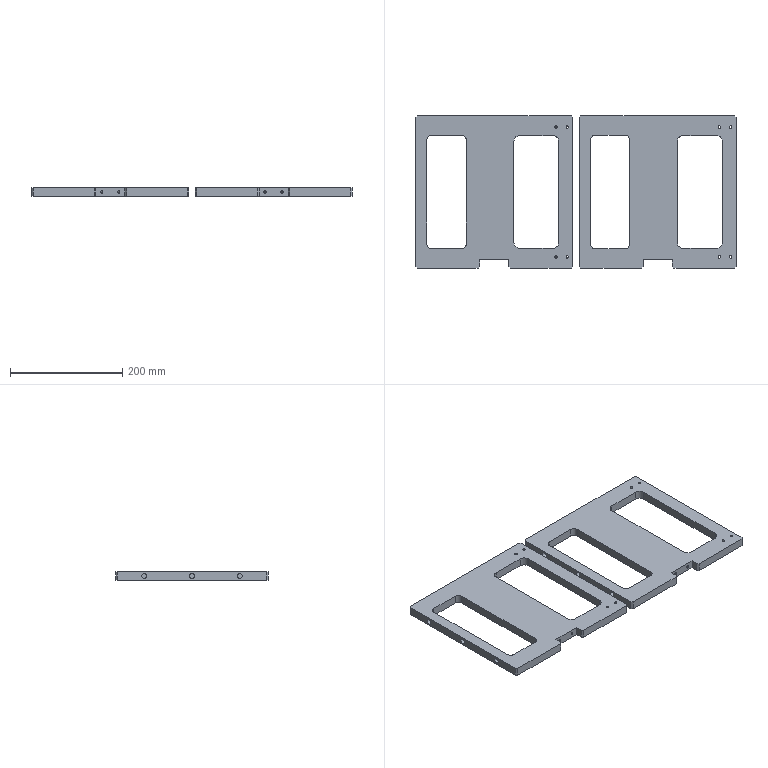Part | 2 solids | 86 faces | box 570 x 271 x 15 mm | volume 1340241 mm3 | plane 48 | cylinder 34 | cone 4 | commonest cylinder face diameters 4.2 x12 16 x8 20 x8 9 x6